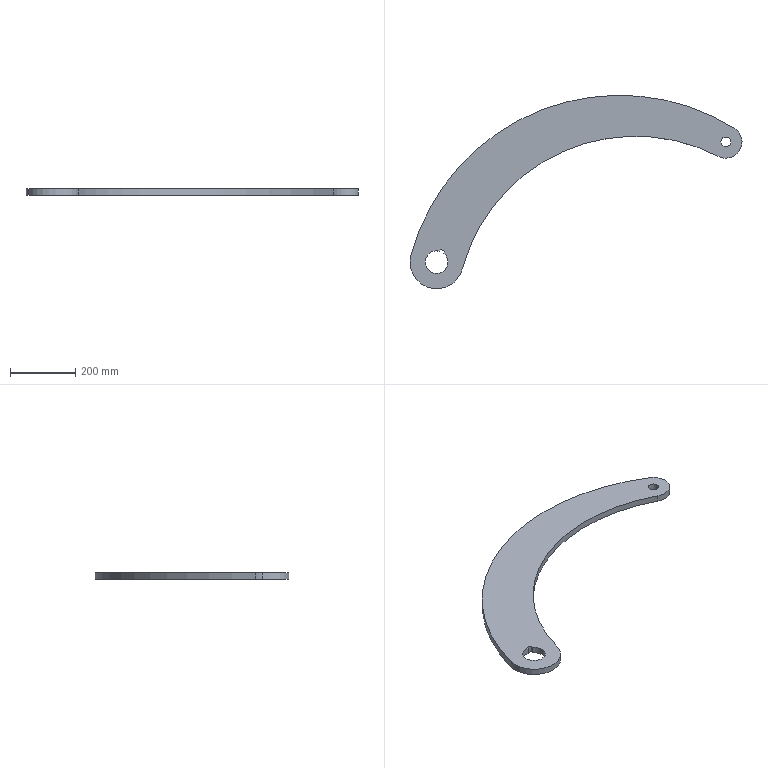Part | SolidWorks | features BaseBody 1 | 1 solid | 15 faces | box 1021 x 595.414 x 20 mm | volume 3303103 mm3 | cylinder 10 | plane 5 | commonest cylinder face diameters 70 x3 30 x2 163.695 x2 100 x1 1105 x1 1331 x1
STEP:
#1=CARTESIAN_POINT('',(3118.424,2172.974,20.));
#2=VERTEX_POINT('',#1);
#3=CARTESIAN_POINT('',(3148.424,2172.974,20.));
#4=VERTEX_POINT('',#3);
#5=CARTESIAN_POINT('',(3133.424,2172.974,20.));
#6=DIRECTION('',(0.,0.,1.));
#7=DIRECTION('',(1.,0.,0.));
#8=AXIS2_PLACEMENT_3D('',#5,#6,#7);
#9=CIRCLE('',#8,15.);
#10=EDGE_CURVE('',#2,#4,#9,.T.);
#11=ORIENTED_EDGE('',*,*,#10,.T.);
#12=CARTESIAN_POINT('',(3148.424,2172.974,0.));
#13=VERTEX_POINT('',#12);
#14=CARTESIAN_POINT('',(3148.424,2172.974,20.));
#15=DIRECTION('',(0.,0.,-1.));
#16=VECTOR('',#15,1000.);
#17=LINE('',#14,#16);
#18=EDGE_CURVE('',#4,#13,#17,.T.);
#19=ORIENTED_EDGE('',*,*,#18,.T.);
#20=CARTESIAN_POINT('',(3118.424,2172.974,0.));
#21=VERTEX_POINT('',#20);
#22=CARTESIAN_POINT('',(3133.424,2172.974,0.));
#23=DIRECTION('',(0.,0.,1.));
#24=DIRECTION('',(1.,0.,0.));
#25=AXIS2_PLACEMENT_3D('',#22,#23,#24);
#26=CIRCLE('',#25,15.);
#27=EDGE_CURVE('',#21,#13,#26,.T.);
#28=ORIENTED_EDGE('',*,*,#27,.F.);
#29=CARTESIAN_POINT('',(3118.424,2172.974,20.));
#30=DIRECTION('',(0.,0.,-1.));
#31=VECTOR('',#30,1000.);
#32=LINE('',#29,#31);
#33=EDGE_CURVE('',#2,#21,#32,.T.);
#34=ORIENTED_EDGE('',*,*,#33,.F.);
#35=EDGE_LOOP('',(#11,#19,#28,#34));
#36=FACE_OUTER_BOUND('',#35,.T.);
#37=CARTESIAN_POINT('',(3133.424,2172.974,20.));
#38=DIRECTION('',(0.,0.,-1.));
#39=DIRECTION('',(-1.,0.,0.));
#40=AXIS2_PLACEMENT_3D('',#37,#38,#39);
#41=CYLINDRICAL_SURFACE('',#40,15.);
#42=ADVANCED_FACE('',(#36),#41,.F.);
#43=CARTESIAN_POINT('',(2208.774,1802.963,20.));
#44=VERTEX_POINT('',#43);
#45=CARTESIAN_POINT('',(2278.774,1802.963,20.));
#46=VERTEX_POINT('',#45);
#47=CARTESIAN_POINT('',(2243.774,1802.963,20.));
#48=DIRECTION('',(0.,0.,1.));
#49=DIRECTION('',(1.,0.,0.));
#50=AXIS2_PLACEMENT_3D('',#47,#48,#49);
#51=CIRCLE('',#50,35.);
#52=EDGE_CURVE('',#44,#46,#51,.T.);
#53=ORIENTED_EDGE('',*,*,#52,.T.);
#54=CARTESIAN_POINT('',(2278.774,1802.963,0.));
#55=VERTEX_POINT('',#54);
#56=CARTESIAN_POINT('',(2278.774,1802.963,20.));
#57=DIRECTION('',(0.,0.,-1.));
#58=VECTOR('',#57,1000.);
#59=LINE('',#56,#58);
#60=EDGE_CURVE('',#46,#55,#59,.T.);
#61=ORIENTED_EDGE('',*,*,#60,.T.);
#62=CARTESIAN_POINT('',(2208.774,1802.963,0.));
#63=VERTEX_POINT('',#62);
#64=CARTESIAN_POINT('',(2243.774,1802.963,0.));
#65=DIRECTION('',(0.,0.,1.));
#66=DIRECTION('',(1.,0.,0.));
#67=AXIS2_PLACEMENT_3D('',#64,#65,#66);
#68=CIRCLE('',#67,35.);
#69=EDGE_CURVE('',#63,#55,#68,.T.);
#70=ORIENTED_EDGE('',*,*,#69,.F.);
#71=CARTESIAN_POINT('',(2208.774,1802.963,20.));
#72=DIRECTION('',(0.,0.,-1.));
#73=VECTOR('',#72,1000.);
#74=LINE('',#71,#73);
#75=EDGE_CURVE('',#44,#63,#74,.T.);
#76=ORIENTED_EDGE('',*,*,#75,.F.);
#77=EDGE_LOOP('',(#53,#61,#70,#76));
#78=FACE_OUTER_BOUND('',#77,.T.);
#79=CARTESIAN_POINT('',(2243.774,1802.963,20.));
#80=DIRECTION('',(0.,0.,-1.));
#81=DIRECTION('',(-1.,0.,0.));
#82=AXIS2_PLACEMENT_3D('',#79,#80,#81);
#83=CYLINDRICAL_SURFACE('',#82,35.);
#84=ADVANCED_FACE('',(#78),#83,.F.);
#85=CARTESIAN_POINT('',(2251.818,1837.026,20.));
#86=VERTEX_POINT('',#85);
#87=CARTESIAN_POINT('',(2243.774,1802.963,20.));
#88=DIRECTION('',(0.,0.,1.));
#89=DIRECTION('',(1.,0.,0.));
#90=AXIS2_PLACEMENT_3D('',#87,#88,#89);
#91=CIRCLE('',#90,35.);
#92=EDGE_CURVE('',#86,#44,#91,.T.);
#93=ORIENTED_EDGE('',*,*,#92,.T.);
#94=ORIENTED_EDGE('',*,*,#75,.T.);
#95=CARTESIAN_POINT('',(2251.818,1837.026,0.));
#96=VERTEX_POINT('',#95);
#97=CARTESIAN_POINT('',(2243.774,1802.963,0.));
#98=DIRECTION('',(0.,0.,1.));
#99=DIRECTION('',(1.,0.,0.));
#100=AXIS2_PLACEMENT_3D('',#97,#98,#99);
#101=CIRCLE('',#100,35.);
#102=EDGE_CURVE('',#96,#63,#101,.T.);
#103=ORIENTED_EDGE('',*,*,#102,.F.);
#104=CARTESIAN_POINT('',(2251.818,1837.026,20.));
#105=DIRECTION('',(0.,0.,-1.));
#106=VECTOR('',#105,1000.);
#107=LINE('',#104,#106);
#108=EDGE_CURVE('',#86,#96,#107,.T.);
#109=ORIENTED_EDGE('',*,*,#108,.F.);
#110=EDGE_LOOP('',(#93,#94,#103,#109));
#111=FACE_OUTER_BOUND('',#110,.T.);
#112=CARTESIAN_POINT('',(2243.774,1802.963,20.));
#113=DIRECTION('',(0.,0.,-1.));
#114=DIRECTION('',(-1.,0.,0.));
#115=AXIS2_PLACEMENT_3D('',#112,#113,#114);
#116=CYLINDRICAL_SURFACE('',#115,35.);
#117=ADVANCED_FACE('',(#111),#116,.F.);
#118=CARTESIAN_POINT('',(2161.927,1802.963,20.));
#119=VERTEX_POINT('',#118);
#120=CARTESIAN_POINT('',(2323.18,1783.12,20.));
#121=VERTEX_POINT('',#120);
#122=CARTESIAN_POINT('',(2243.774,1802.963,20.));
#123=DIRECTION('',(0.,0.,1.));
#124=DIRECTION('',(1.,0.,0.));
#125=AXIS2_PLACEMENT_3D('',#122,#123,#124);
#126=CIRCLE('',#125,81.847);
#127=EDGE_CURVE('',#119,#121,#126,.T.);
#128=ORIENTED_EDGE('',*,*,#127,.F.);
#129=CARTESIAN_POINT('',(2161.927,1802.963,0.));
#130=VERTEX_POINT('',#129);
#131=CARTESIAN_POINT('',(2161.927,1802.963,20.));
#132=DIRECTION('',(0.,0.,-1.));
#133=VECTOR('',#132,1000.);
#134=LINE('',#131,#133);
#135=EDGE_CURVE('',#119,#130,#134,.T.);
#136=ORIENTED_EDGE('',*,*,#135,.T.);
#137=CARTESIAN_POINT('',(2323.18,1783.12,0.));
#138=VERTEX_POINT('',#137);
#139=CARTESIAN_POINT('',(2243.774,1802.963,0.));
#140=DIRECTION('',(0.,0.,1.));
#141=DIRECTION('',(1.,0.,0.));
#142=AXIS2_PLACEMENT_3D('',#139,#140,#141);
#143=CIRCLE('',#142,81.847);
#144=EDGE_CURVE('',#130,#138,#143,.T.);
#145=ORIENTED_EDGE('',*,*,#144,.T.);
#146=CARTESIAN_POINT('',(2323.18,1783.12,20.));
#147=DIRECTION('',(0.,0.,-1.));
#148=VECTOR('',#147,1000.);
#149=LINE('',#146,#148);
#150=EDGE_CURVE('',#121,#138,#149,.T.);
#151=ORIENTED_EDGE('',*,*,#150,.F.);
#152=EDGE_LOOP('',(#128,#136,#145,#151));
#153=FACE_OUTER_BOUND('',#152,.T.);
#154=CARTESIAN_POINT('',(2243.774,1802.963,20.));
#155=DIRECTION('',(0.,0.,-1.));
#156=DIRECTION('',(-1.,0.,0.));
#157=AXIS2_PLACEMENT_3D('',#154,#155,#156);
#158=CYLINDRICAL_SURFACE('',#157,81.847);
#159=ADVANCED_FACE('',(#153),#158,.T.);
#160=CARTESIAN_POINT('',(3161.406,2214.411,0.));
#161=VERTEX_POINT('',#160);
#162=CARTESIAN_POINT('',(2164.511,1823.366,0.));
#163=VERTEX_POINT('',#162);
#164=CARTESIAN_POINT('',(2807.2,1651.173,0.));
#165=DIRECTION('',(0.,0.,1.));
#166=DIRECTION('',(1.,0.,0.));
#167=AXIS2_PLACEMENT_3D('',#164,#165,#166);
#168=CIRCLE('',#167,665.357);
#169=EDGE_CURVE('',#161,#163,#168,.T.);
#170=ORIENTED_EDGE('',*,*,#169,.T.);
#171=CARTESIAN_POINT('',(2164.511,1823.366,20.));
#172=VERTEX_POINT('',#171);
#173=CARTESIAN_POINT('',(2164.511,1823.366,20.));
#174=DIRECTION('',(0.,0.,-1.));
#175=VECTOR('',#174,1000.);
#176=LINE('',#173,#175);
#177=EDGE_CURVE('',#172,#163,#176,.T.);
#178=ORIENTED_EDGE('',*,*,#177,.F.);
#179=CARTESIAN_POINT('',(3161.406,2214.411,20.));
#180=VERTEX_POINT('',#179);
#181=CARTESIAN_POINT('',(2807.2,1651.173,20.));
#182=DIRECTION('',(0.,0.,1.));
#183=DIRECTION('',(1.,0.,0.));
#184=AXIS2_PLACEMENT_3D('',#181,#182,#183);
#185=CIRCLE('',#184,665.357);
#186=EDGE_CURVE('',#180,#172,#185,.T.);
#187=ORIENTED_EDGE('',*,*,#186,.F.);
#188=CARTESIAN_POINT('',(3161.406,2214.411,20.));
#189=DIRECTION('',(0.,0.,-1.));
#190=VECTOR('',#189,1000.);
#191=LINE('',#188,#190);
#192=EDGE_CURVE('',#180,#161,#191,.T.);
#193=ORIENTED_EDGE('',*,*,#192,.T.);
#194=EDGE_LOOP('',(#170,#178,#187,#193));
#195=FACE_OUTER_BOUND('',#194,.T.);
#196=CARTESIAN_POINT('',(2807.2,1651.173,20.));
#197=DIRECTION('',(0.,0.,-1.));
#198=DIRECTION('',(-1.,0.,0.));
#199=AXIS2_PLACEMENT_3D('',#196,#197,#198);
#200=CYLINDRICAL_SURFACE('',#199,665.357);
#201=ADVANCED_FACE('',(#195),#200,.T.);
#202=ORIENTED_EDGE('',*,*,#135,.F.);
#203=CARTESIAN_POINT('',(2243.774,1802.963,20.));
#204=DIRECTION('',(0.,0.,1.));
#205=DIRECTION('',(1.,0.,0.));
#206=AXIS2_PLACEMENT_3D('',#203,#204,#205);
#207=CIRCLE('',#206,81.847);
#208=EDGE_CURVE('',#172,#119,#207,.T.);
#209=ORIENTED_EDGE('',*,*,#208,.F.);
#210=ORIENTED_EDGE('',*,*,#177,.T.);
#211=CARTESIAN_POINT('',(2243.774,1802.963,0.));
#212=DIRECTION('',(0.,0.,1.));
#213=DIRECTION('',(1.,0.,0.));
#214=AXIS2_PLACEMENT_3D('',#211,#212,#213);
#215=CIRCLE('',#214,81.847);
#216=EDGE_CURVE('',#163,#130,#215,.T.);
#217=ORIENTED_EDGE('',*,*,#216,.T.);
#218=EDGE_LOOP('',(#202,#209,#210,#217));
#219=FACE_OUTER_BOUND('',#218,.T.);
#220=CARTESIAN_POINT('',(2243.774,1802.963,20.));
#221=DIRECTION('',(0.,0.,-1.));
#222=DIRECTION('',(-1.,0.,0.));
#223=AXIS2_PLACEMENT_3D('',#220,#221,#222);
#224=CYLINDRICAL_SURFACE('',#223,81.847);
#225=ADVANCED_FACE('',(#219),#224,.T.);
#226=CARTESIAN_POINT('',(3109.383,2129.134,0.));
#227=VERTEX_POINT('',#226);
#228=CARTESIAN_POINT('',(2856.193,1638.223,0.));
#229=DIRECTION('',(0.,0.,1.));
#230=DIRECTION('',(1.,0.,0.));
#231=AXIS2_PLACEMENT_3D('',#228,#229,#230);
#232=CIRCLE('',#231,552.357);
#233=EDGE_CURVE('',#227,#138,#232,.T.);
#234=ORIENTED_EDGE('',*,*,#233,.F.);
#235=CARTESIAN_POINT('',(3109.383,2129.134,20.));
#236=VERTEX_POINT('',#235);
#237=CARTESIAN_POINT('',(3109.383,2129.134,20.));
#238=DIRECTION('',(0.,0.,-1.));
#239=VECTOR('',#238,1000.);
#240=LINE('',#237,#239);
#241=EDGE_CURVE('',#236,#227,#240,.T.);
#242=ORIENTED_EDGE('',*,*,#241,.F.);
#243=CARTESIAN_POINT('',(2856.193,1638.223,20.));
#244=DIRECTION('',(0.,0.,1.));
#245=DIRECTION('',(1.,0.,0.));
#246=AXIS2_PLACEMENT_3D('',#243,#244,#245);
#247=CIRCLE('',#246,552.357);
#248=EDGE_CURVE('',#236,#121,#247,.T.);
#249=ORIENTED_EDGE('',*,*,#248,.T.);
#250=ORIENTED_EDGE('',*,*,#150,.T.);
#251=EDGE_LOOP('',(#234,#242,#249,#250));
#252=FACE_OUTER_BOUND('',#251,.T.);
#253=CARTESIAN_POINT('',(2856.193,1638.223,20.));
#254=DIRECTION('',(0.,0.,-1.));
#255=DIRECTION('',(-1.,0.,0.));
#256=AXIS2_PLACEMENT_3D('',#253,#254,#255);
#257=CYLINDRICAL_SURFACE('',#256,552.357);
#258=ADVANCED_FACE('',(#252),#257,.F.);
#259=ORIENTED_EDGE('',*,*,#60,.F.);
#260=CARTESIAN_POINT('',(2264.525,1831.148,20.));
#261=VERTEX_POINT('',#260);
#262=CARTESIAN_POINT('',(2243.774,1802.963,20.));
#263=DIRECTION('',(0.,0.,1.));
#264=DIRECTION('',(1.,0.,0.));
#265=AXIS2_PLACEMENT_3D('',#262,#263,#264);
#266=CIRCLE('',#265,35.);
#267=EDGE_CURVE('',#46,#261,#266,.T.);
#268=ORIENTED_EDGE('',*,*,#267,.T.);
#269=CARTESIAN_POINT('',(2264.525,1831.148,0.));
#270=VERTEX_POINT('',#269);
#271=CARTESIAN_POINT('',(2264.525,1831.148,20.));
#272=DIRECTION('',(0.,0.,-1.));
#273=VECTOR('',#272,1000.);
#274=LINE('',#271,#273);
#275=EDGE_CURVE('',#261,#270,#274,.T.);
#276=ORIENTED_EDGE('',*,*,#275,.T.);
#277=CARTESIAN_POINT('',(2243.774,1802.963,0.));
#278=DIRECTION('',(0.,0.,1.));
#279=DIRECTION('',(1.,0.,0.));
#280=AXIS2_PLACEMENT_3D('',#277,#278,#279);
#281=CIRCLE('',#280,35.);
#282=EDGE_CURVE('',#55,#270,#281,.T.);
#283=ORIENTED_EDGE('',*,*,#282,.F.);
#284=EDGE_LOOP('',(#259,#268,#276,#283));
#285=FACE_OUTER_BOUND('',#284,.T.);
#286=CARTESIAN_POINT('',(2243.774,1802.963,20.));
#287=DIRECTION('',(0.,0.,-1.));
#288=DIRECTION('',(-1.,0.,0.));
#289=AXIS2_PLACEMENT_3D('',#286,#287,#288);
#290=CYLINDRICAL_SURFACE('',#289,35.);
#291=ADVANCED_FACE('',(#285),#290,.F.);
#292=CARTESIAN_POINT('',(2254.634,1843.113,0.));
#293=VERTEX_POINT('',#292);
#294=CARTESIAN_POINT('',(1154.904,-534.242,0.));
#295=DIRECTION('',(-0.4198,-0.9076,0.));
#296=VECTOR('',#295,1000.);
#297=LINE('',#294,#296);
#298=EDGE_CURVE('',#293,#96,#297,.T.);
#299=ORIENTED_EDGE('',*,*,#298,.F.);
#300=CARTESIAN_POINT('',(2254.634,1843.113,20.));
#301=VERTEX_POINT('',#300);
#302=CARTESIAN_POINT('',(2254.634,1843.113,20.));
#303=DIRECTION('',(0.,0.,-1.));
#304=VECTOR('',#303,1000.);
#305=LINE('',#302,#304);
#306=EDGE_CURVE('',#301,#293,#305,.T.);
#307=ORIENTED_EDGE('',*,*,#306,.F.);
#308=CARTESIAN_POINT('',(1154.904,-534.242,20.));
#309=DIRECTION('',(-0.4198,-0.9076,0.));
#310=VECTOR('',#309,1000.);
#311=LINE('',#308,#310);
#312=EDGE_CURVE('',#301,#86,#311,.T.);
#313=ORIENTED_EDGE('',*,*,#312,.T.);
#314=ORIENTED_EDGE('',*,*,#108,.T.);
#315=EDGE_LOOP('',(#299,#307,#313,#314));
#316=FACE_OUTER_BOUND('',#315,.T.);
#317=CARTESIAN_POINT('',(1154.904,-534.242,20.));
#318=DIRECTION('',(0.9076,-0.4198,0.));
#319=DIRECTION('',(0.4198,0.9076,0.));
#320=AXIS2_PLACEMENT_3D('',#317,#318,#319);
#321=PLANE('',#320);
#322=ADVANCED_FACE('',(#316),#321,.T.);
#323=CARTESIAN_POINT('',(2267.341,1837.235,0.));
#324=VERTEX_POINT('',#323);
#325=CARTESIAN_POINT('',(1099.73,2377.355,0.));
#326=DIRECTION('',(0.9076,-0.4198,0.));
#327=VECTOR('',#326,1000.);
#328=LINE('',#325,#327);
#329=EDGE_CURVE('',#293,#324,#328,.T.);
#330=ORIENTED_EDGE('',*,*,#329,.T.);
#331=CARTESIAN_POINT('',(2267.341,1837.235,20.));
#332=VERTEX_POINT('',#331);
#333=CARTESIAN_POINT('',(2267.341,1837.235,20.));
#334=DIRECTION('',(0.,0.,-1.));
#335=VECTOR('',#334,1000.);
#336=LINE('',#333,#335);
#337=EDGE_CURVE('',#332,#324,#336,.T.);
#338=ORIENTED_EDGE('',*,*,#337,.F.);
#339=CARTESIAN_POINT('',(1099.73,2377.355,20.));
#340=DIRECTION('',(0.9076,-0.4198,0.));
#341=VECTOR('',#340,1000.);
#342=LINE('',#339,#341);
#343=EDGE_CURVE('',#301,#332,#342,.T.);
#344=ORIENTED_EDGE('',*,*,#343,.F.);
#345=ORIENTED_EDGE('',*,*,#306,.T.);
#346=EDGE_LOOP('',(#330,#338,#344,#345));
#347=FACE_OUTER_BOUND('',#346,.T.);
#348=CARTESIAN_POINT('',(1099.73,2377.355,20.));
#349=DIRECTION('',(0.4198,0.9076,0.));
#350=DIRECTION('',(-0.9076,0.4198,0.));
#351=AXIS2_PLACEMENT_3D('',#348,#349,#350);
#352=PLANE('',#351);
#353=ADVANCED_FACE('',(#347),#352,.F.);
#354=CARTESIAN_POINT('',(1167.61,-540.12,0.));
#355=DIRECTION('',(-0.4198,-0.9076,0.));
#356=VECTOR('',#355,1000.);
#357=LINE('',#354,#356);
#358=EDGE_CURVE('',#324,#270,#357,.T.);
#359=ORIENTED_EDGE('',*,*,#358,.T.);
#360=ORIENTED_EDGE('',*,*,#275,.F.);
#361=CARTESIAN_POINT('',(1167.61,-540.12,20.));
#362=DIRECTION('',(-0.4198,-0.9076,0.));
#363=VECTOR('',#362,1000.);
#364=LINE('',#361,#363);
#365=EDGE_CURVE('',#332,#261,#364,.T.);
#366=ORIENTED_EDGE('',*,*,#365,.F.);
#367=ORIENTED_EDGE('',*,*,#337,.T.);
#368=EDGE_LOOP('',(#359,#360,#366,#367));
#369=FACE_OUTER_BOUND('',#368,.T.);
#370=CARTESIAN_POINT('',(1167.61,-540.12,20.));
#371=DIRECTION('',(0.9076,-0.4198,0.));
#372=DIRECTION('',(0.4198,0.9076,0.));
#373=AXIS2_PLACEMENT_3D('',#370,#371,#372);
#374=PLANE('',#373);
#375=ADVANCED_FACE('',(#369),#374,.F.);
#376=ORIENTED_EDGE('',*,*,#18,.F.);
#377=CARTESIAN_POINT('',(3133.424,2172.974,20.));
#378=DIRECTION('',(0.,0.,1.));
#379=DIRECTION('',(1.,0.,0.));
#380=AXIS2_PLACEMENT_3D('',#377,#378,#379);
#381=CIRCLE('',#380,15.);
#382=EDGE_CURVE('',#4,#2,#381,.T.);
#383=ORIENTED_EDGE('',*,*,#382,.T.);
#384=ORIENTED_EDGE('',*,*,#33,.T.);
#385=CARTESIAN_POINT('',(3133.424,2172.974,0.));
#386=DIRECTION('',(0.,0.,1.));
#387=DIRECTION('',(1.,0.,0.));
#388=AXIS2_PLACEMENT_3D('',#385,#386,#387);
#389=CIRCLE('',#388,15.);
#390=EDGE_CURVE('',#13,#21,#389,.T.);
#391=ORIENTED_EDGE('',*,*,#390,.F.);
#392=EDGE_LOOP('',(#376,#383,#384,#391));
#393=FACE_OUTER_BOUND('',#392,.T.);
#394=CARTESIAN_POINT('',(3133.424,2172.974,20.));
#395=DIRECTION('',(0.,0.,-1.));
#396=DIRECTION('',(-1.,0.,0.));
#397=AXIS2_PLACEMENT_3D('',#394,#395,#396);
#398=CYLINDRICAL_SURFACE('',#397,15.);
#399=ADVANCED_FACE('',(#393),#398,.F.);
#400=CARTESIAN_POINT('',(3133.424,2172.974,0.));
#401=DIRECTION('',(0.,0.,1.));
#402=DIRECTION('',(1.,0.,0.));
#403=AXIS2_PLACEMENT_3D('',#400,#401,#402);
#404=CIRCLE('',#403,50.);
#405=EDGE_CURVE('',#227,#161,#404,.T.);
#406=ORIENTED_EDGE('',*,*,#405,.T.);
#407=ORIENTED_EDGE('',*,*,#192,.F.);
#408=CARTESIAN_POINT('',(3133.424,2172.974,20.));
#409=DIRECTION('',(0.,0.,1.));
#410=DIRECTION('',(1.,0.,0.));
#411=AXIS2_PLACEMENT_3D('',#408,#409,#410);
#412=CIRCLE('',#411,50.);
#413=EDGE_CURVE('',#236,#180,#412,.T.);
#414=ORIENTED_EDGE('',*,*,#413,.F.);
#415=ORIENTED_EDGE('',*,*,#241,.T.);
#416=EDGE_LOOP('',(#406,#407,#414,#415));
#417=FACE_OUTER_BOUND('',#416,.T.);
#418=CARTESIAN_POINT('',(3133.424,2172.974,20.));
#419=DIRECTION('',(0.,0.,-1.));
#420=DIRECTION('',(-1.,0.,0.));
#421=AXIS2_PLACEMENT_3D('',#418,#419,#420);
#422=CYLINDRICAL_SURFACE('',#421,50.);
#423=ADVANCED_FACE('',(#417),#422,.T.);
#424=ORIENTED_EDGE('',*,*,#10,.F.);
#425=ORIENTED_EDGE('',*,*,#382,.F.);
#426=EDGE_LOOP('',(#424,#425));
#427=FACE_BOUND('',#426,.T.);
#428=ORIENTED_EDGE('',*,*,#92,.F.);
#429=ORIENTED_EDGE('',*,*,#312,.F.);
#430=ORIENTED_EDGE('',*,*,#343,.T.);
#431=ORIENTED_EDGE('',*,*,#365,.T.);
#432=ORIENTED_EDGE('',*,*,#267,.F.);
#433=ORIENTED_EDGE('',*,*,#52,.F.);
#434=EDGE_LOOP('',(#428,#429,#430,#431,#432,#433));
#435=FACE_BOUND('',#434,.T.);
#436=ORIENTED_EDGE('',*,*,#186,.T.);
#437=ORIENTED_EDGE('',*,*,#208,.T.);
#438=ORIENTED_EDGE('',*,*,#127,.T.);
#439=ORIENTED_EDGE('',*,*,#248,.F.);
#440=ORIENTED_EDGE('',*,*,#413,.T.);
#441=EDGE_LOOP('',(#436,#437,#438,#439,#440));
#442=FACE_OUTER_BOUND('',#441,.T.);
#443=CARTESIAN_POINT('',(0.,0.,20.));
#444=DIRECTION('',(0.,0.,1.));
#445=DIRECTION('',(1.,0.,0.));
#446=AXIS2_PLACEMENT_3D('',#443,#444,#445);
#447=PLANE('',#446);
#448=ADVANCED_FACE('',(#427,#435,#442),#447,.T.);
#449=ORIENTED_EDGE('',*,*,#27,.T.);
#450=ORIENTED_EDGE('',*,*,#390,.T.);
#451=EDGE_LOOP('',(#449,#450));
#452=FACE_BOUND('',#451,.T.);
#453=ORIENTED_EDGE('',*,*,#102,.T.);
#454=ORIENTED_EDGE('',*,*,#69,.T.);
#455=ORIENTED_EDGE('',*,*,#282,.T.);
#456=ORIENTED_EDGE('',*,*,#358,.F.);
#457=ORIENTED_EDGE('',*,*,#329,.F.);
#458=ORIENTED_EDGE('',*,*,#298,.T.);
#459=EDGE_LOOP('',(#453,#454,#455,#456,#457,#458));
#460=FACE_BOUND('',#459,.T.);
#461=ORIENTED_EDGE('',*,*,#169,.F.);
#462=ORIENTED_EDGE('',*,*,#405,.F.);
#463=ORIENTED_EDGE('',*,*,#233,.T.);
#464=ORIENTED_EDGE('',*,*,#144,.F.);
#465=ORIENTED_EDGE('',*,*,#216,.F.);
#466=EDGE_LOOP('',(#461,#462,#463,#464,#465));
#467=FACE_OUTER_BOUND('',#466,.T.);
#468=CARTESIAN_POINT('',(0.,0.,0.));
#469=DIRECTION('',(0.,0.,1.));
#470=DIRECTION('',(1.,0.,0.));
#471=AXIS2_PLACEMENT_3D('',#468,#469,#470);
#472=PLANE('',#471);
#473=ADVANCED_FACE('',(#452,#460,#467),#472,.F.);
#474=CLOSED_SHELL('',(#42,#84,#117,#159,#201,#225,#258,#291,#322,#353,#375,#399,#423,#448,#473));
#475=MANIFOLD_SOLID_BREP('',#474);
#476=CARTESIAN_POINT('',(0.,0.,0.));
#477=DIRECTION('',(0.,0.,1.));
#478=DIRECTION('',(1.,0.,0.));
#479=AXIS2_PLACEMENT_3D('',#476,#477,#478);
#480=(LENGTH_UNIT()NAMED_UNIT(*)SI_UNIT(.MILLI.,.METRE.));
#481=UNCERTAINTY_MEASURE_WITH_UNIT(LENGTH_MEASURE(0.00001),#480,'','');
#482=(NAMED_UNIT(*)PLANE_ANGLE_UNIT()SI_UNIT($,.RADIAN.));
#483=(NAMED_UNIT(*)SI_UNIT($,.STERADIAN.)SOLID_ANGLE_UNIT());
#484=(GEOMETRIC_REPRESENTATION_CONTEXT(3)GLOBAL_UNCERTAINTY_ASSIGNED_CONTEXT((#481))GLOBAL_UNIT_ASSIGNED_CONTEXT((#480,#482,#483))REPRESENTATION_CONTEXT('',''));
#485=ADVANCED_BREP_SHAPE_REPRESENTATION('',(#475,#479),#484);